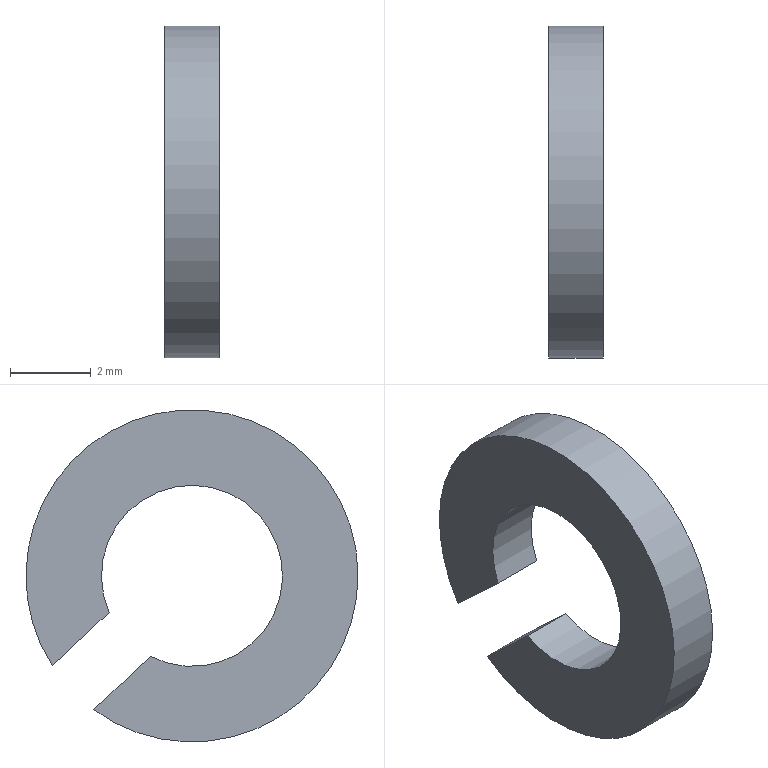Part | NX | features TAM02-M3-L8-002 2 | 1 solid | 6 faces | box 1.35 x 8.25 x 8.25 mm | volume 46.859 mm3 | plane 4 | cylinder 2 | commonest cylinder face diameters 4.5 x1 8.25 x1
STEP:
#1=CARTESIAN_POINT('',(131.823,-41.668,-38.5));
#2=VERTEX_POINT('',#1);
#3=CARTESIAN_POINT('',(131.823,-40.641,-37.407));
#4=VERTEX_POINT('',#3);
#5=CARTESIAN_POINT('',(131.823,-42.7,-36.5));
#6=DIRECTION('',(1.,0.,0.));
#7=DIRECTION('',(0.,0.9152,-0.403));
#8=AXIS2_PLACEMENT_3D('',#5,#6,#7);
#9=CIRCLE('',#8,2.25);
#10=EDGE_CURVE('',#2,#4,#9,.F.);
#11=ORIENTED_EDGE('',*,*,#10,.T.);
#12=CARTESIAN_POINT('',(133.173,-40.641,-37.407));
#13=VERTEX_POINT('',#12);
#14=CARTESIAN_POINT('',(131.823,-40.641,-37.407));
#15=DIRECTION('',(1.,0.,0.));
#16=VECTOR('',#15,1000.);
#17=LINE('',#14,#16);
#18=EDGE_CURVE('',#13,#4,#17,.F.);
#19=ORIENTED_EDGE('',*,*,#18,.F.);
#20=CARTESIAN_POINT('',(133.173,-41.668,-38.5));
#21=VERTEX_POINT('',#20);
#22=CARTESIAN_POINT('',(133.173,-42.7,-36.5));
#23=DIRECTION('',(1.,0.,0.));
#24=DIRECTION('',(0.,0.9152,-0.403));
#25=AXIS2_PLACEMENT_3D('',#22,#23,#24);
#26=CIRCLE('',#25,2.25);
#27=EDGE_CURVE('',#21,#13,#26,.F.);
#28=ORIENTED_EDGE('',*,*,#27,.F.);
#29=CARTESIAN_POINT('',(131.823,-41.668,-38.5));
#30=DIRECTION('',(1.,0.,0.));
#31=VECTOR('',#30,1000.);
#32=LINE('',#29,#31);
#33=EDGE_CURVE('',#21,#2,#32,.F.);
#34=ORIENTED_EDGE('',*,*,#33,.T.);
#35=EDGE_LOOP('',(#11,#19,#28,#34));
#36=FACE_BOUND('',#35,.T.);
#37=CARTESIAN_POINT('',(131.823,-42.7,-36.5));
#38=DIRECTION('',(1.,0.,0.));
#39=DIRECTION('',(0.,0.7285,-0.685));
#40=AXIS2_PLACEMENT_3D('',#37,#38,#39);
#41=CYLINDRICAL_SURFACE('',#40,2.25);
#42=ADVANCED_FACE('',(#36),#41,.F.);
#43=CARTESIAN_POINT('',(131.823,-40.259,-39.825));
#44=VERTEX_POINT('',#43);
#45=CARTESIAN_POINT('',(131.823,-39.231,-38.732));
#46=VERTEX_POINT('',#45);
#47=CARTESIAN_POINT('',(131.823,-42.7,-36.5));
#48=DIRECTION('',(1.,0.,0.));
#49=DIRECTION('',(0.,0.8409,-0.5411));
#50=AXIS2_PLACEMENT_3D('',#47,#48,#49);
#51=CIRCLE('',#50,4.125);
#52=EDGE_CURVE('',#44,#46,#51,.F.);
#53=ORIENTED_EDGE('',*,*,#52,.F.);
#54=CARTESIAN_POINT('',(133.173,-40.259,-39.825));
#55=VERTEX_POINT('',#54);
#56=CARTESIAN_POINT('',(131.823,-40.259,-39.825));
#57=DIRECTION('',(1.,0.,0.));
#58=VECTOR('',#57,1000.);
#59=LINE('',#56,#58);
#60=EDGE_CURVE('',#55,#44,#59,.F.);
#61=ORIENTED_EDGE('',*,*,#60,.F.);
#62=CARTESIAN_POINT('',(133.173,-39.231,-38.732));
#63=VERTEX_POINT('',#62);
#64=CARTESIAN_POINT('',(133.173,-42.7,-36.5));
#65=DIRECTION('',(1.,0.,0.));
#66=DIRECTION('',(0.,0.8409,-0.5411));
#67=AXIS2_PLACEMENT_3D('',#64,#65,#66);
#68=CIRCLE('',#67,4.125);
#69=EDGE_CURVE('',#55,#63,#68,.F.);
#70=ORIENTED_EDGE('',*,*,#69,.T.);
#71=CARTESIAN_POINT('',(131.823,-39.231,-38.732));
#72=DIRECTION('',(1.,0.,0.));
#73=VECTOR('',#72,1000.);
#74=LINE('',#71,#73);
#75=EDGE_CURVE('',#63,#46,#74,.F.);
#76=ORIENTED_EDGE('',*,*,#75,.T.);
#77=EDGE_LOOP('',(#53,#61,#70,#76));
#78=FACE_BOUND('',#77,.T.);
#79=CARTESIAN_POINT('',(131.823,-42.7,-36.5));
#80=DIRECTION('',(1.,0.,0.));
#81=DIRECTION('',(0.,0.7285,-0.685));
#82=AXIS2_PLACEMENT_3D('',#79,#80,#81);
#83=CYLINDRICAL_SURFACE('',#82,4.125);
#84=ADVANCED_FACE('',(#78),#83,.T.);
#85=CARTESIAN_POINT('',(133.173,-40.641,-37.407));
#86=DIRECTION('',(0.,0.7285,-0.685));
#87=VECTOR('',#86,1000.);
#88=LINE('',#85,#87);
#89=EDGE_CURVE('',#63,#13,#88,.F.);
#90=ORIENTED_EDGE('',*,*,#89,.T.);
#91=ORIENTED_EDGE('',*,*,#18,.T.);
#92=CARTESIAN_POINT('',(131.823,-40.641,-37.407));
#93=DIRECTION('',(0.,0.7285,-0.685));
#94=VECTOR('',#93,1000.);
#95=LINE('',#92,#94);
#96=EDGE_CURVE('',#46,#4,#95,.F.);
#97=ORIENTED_EDGE('',*,*,#96,.F.);
#98=ORIENTED_EDGE('',*,*,#75,.F.);
#99=EDGE_LOOP('',(#90,#91,#97,#98));
#100=FACE_BOUND('',#99,.T.);
#101=CARTESIAN_POINT('',(131.823,-40.641,-37.407));
#102=DIRECTION('',(0.,0.685,0.7285));
#103=DIRECTION('',(0.,0.7285,-0.685));
#104=AXIS2_PLACEMENT_3D('',#101,#102,#103);
#105=PLANE('',#104);
#106=ADVANCED_FACE('',(#100),#105,.F.);
#107=CARTESIAN_POINT('',(133.173,-40.259,-39.825));
#108=DIRECTION('',(0.,-0.7285,0.685));
#109=VECTOR('',#108,1000.);
#110=LINE('',#107,#109);
#111=EDGE_CURVE('',#21,#55,#110,.F.);
#112=ORIENTED_EDGE('',*,*,#111,.T.);
#113=ORIENTED_EDGE('',*,*,#60,.T.);
#114=CARTESIAN_POINT('',(131.823,-40.259,-39.825));
#115=DIRECTION('',(0.,-0.7285,0.685));
#116=VECTOR('',#115,1000.);
#117=LINE('',#114,#116);
#118=EDGE_CURVE('',#2,#44,#117,.F.);
#119=ORIENTED_EDGE('',*,*,#118,.F.);
#120=ORIENTED_EDGE('',*,*,#33,.F.);
#121=EDGE_LOOP('',(#112,#113,#119,#120));
#122=FACE_BOUND('',#121,.T.);
#123=CARTESIAN_POINT('',(131.823,-40.259,-39.825));
#124=DIRECTION('',(0.,-0.685,-0.7285));
#125=DIRECTION('',(0.,-0.7285,0.685));
#126=AXIS2_PLACEMENT_3D('',#123,#124,#125);
#127=PLANE('',#126);
#128=ADVANCED_FACE('',(#122),#127,.F.);
#129=ORIENTED_EDGE('',*,*,#96,.T.);
#130=ORIENTED_EDGE('',*,*,#10,.F.);
#131=ORIENTED_EDGE('',*,*,#118,.T.);
#132=ORIENTED_EDGE('',*,*,#52,.T.);
#133=EDGE_LOOP('',(#129,#130,#131,#132));
#134=FACE_BOUND('',#133,.T.);
#135=CARTESIAN_POINT('',(131.823,-42.7,-36.5));
#136=DIRECTION('',(-1.,0.,0.));
#137=DIRECTION('',(0.,-0.7285,0.685));
#138=AXIS2_PLACEMENT_3D('',#135,#136,#137);
#139=PLANE('',#138);
#140=ADVANCED_FACE('',(#134),#139,.T.);
#141=ORIENTED_EDGE('',*,*,#89,.F.);
#142=ORIENTED_EDGE('',*,*,#69,.F.);
#143=ORIENTED_EDGE('',*,*,#111,.F.);
#144=ORIENTED_EDGE('',*,*,#27,.T.);
#145=EDGE_LOOP('',(#141,#142,#143,#144));
#146=FACE_BOUND('',#145,.T.);
#147=CARTESIAN_POINT('',(133.173,-42.7,-36.5));
#148=DIRECTION('',(-1.,0.,0.));
#149=DIRECTION('',(0.,-0.7285,0.685));
#150=AXIS2_PLACEMENT_3D('',#147,#148,#149);
#151=PLANE('',#150);
#152=ADVANCED_FACE('',(#146),#151,.F.);
#153=CLOSED_SHELL('',(#42,#84,#106,#128,#140,#152));
#154=MANIFOLD_SOLID_BREP('',#153);
#155=(LENGTH_UNIT()NAMED_UNIT(*)SI_UNIT(.MILLI.,.METRE.));
#156=UNCERTAINTY_MEASURE_WITH_UNIT(LENGTH_MEASURE(0.00001),#155,'','');
#157=(NAMED_UNIT(*)PLANE_ANGLE_UNIT()SI_UNIT($,.RADIAN.));
#158=(NAMED_UNIT(*)SI_UNIT($,.STERADIAN.)SOLID_ANGLE_UNIT());
#159=(GEOMETRIC_REPRESENTATION_CONTEXT(3)GLOBAL_UNCERTAINTY_ASSIGNED_CONTEXT((#156))GLOBAL_UNIT_ASSIGNED_CONTEXT((#155,#157,#158))REPRESENTATION_CONTEXT('',''));
#160=ADVANCED_BREP_SHAPE_REPRESENTATION('',(#154),#159);